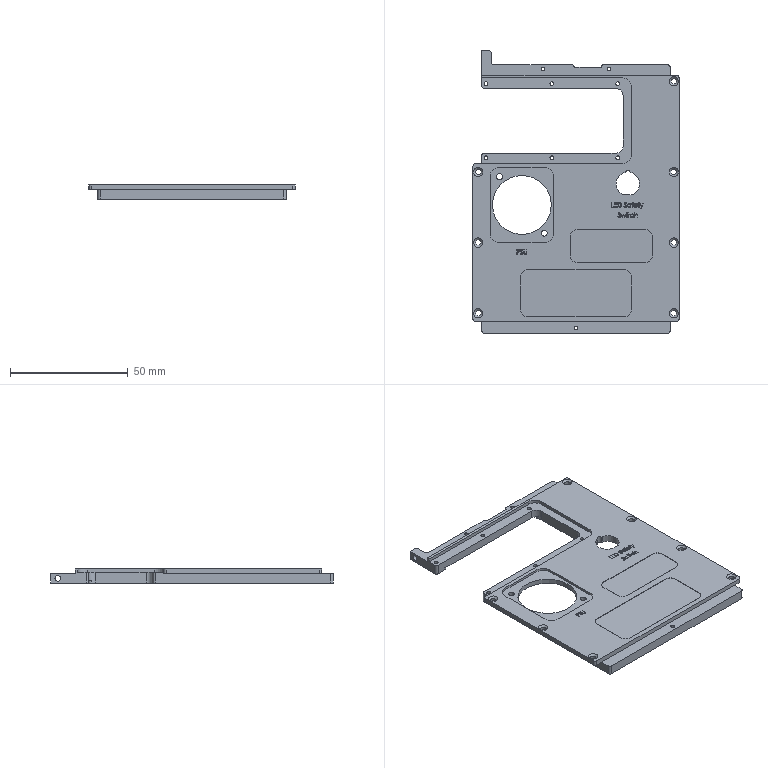NC program | NX | posted with a generic post | part box 87.5 x 120 x 6.001 mm
Whole program:
N10 G17 G21 G94 G90
(PLANAR_MILL_8 , TOOL : D6-18-D6-50-3T-FINISH)
N12 T05 M6
N14 G54
N16 G17 G0 G90 X-15.174 Y-1.985 B0. C0. S5000 M3
N18 G43 Z50. H5
N20 Z-0.75 B-180. C90.
N22 G94 G1 Z-3.75 F300.
N24 G41 X-15. Y-1. D5
N26 Y4.
N28 Y6.
N30 Y11.
N32 G40
N34 X-15.174 Y11.985
N36 Z-0.75
N38 G0 Z50.
N40 M5
(SPOT_DRILLING_3 , TOOL : 点孔D5-120-90度)
N42 T14 M6
N44 G54
N46 G17 G0 G90 X-57. Y2. B0. C0. S2500 M3
N48 G43 Z50. H14
N50 G94 G82 G99 Z-5. B-180. C90. F200. P200 R-0.75
N52 G80
N54 G0 X-57. Y2. Z50.
N56 M5
(SPOT_DRILLING_3_COPY , TOOL : Z2.4)
N58 T15 M6
N60 G54
N62 G17 G0 G90 X-57. Y2. B0. C0. S2500 M3
N64 G43 Z50. H15
N66 G94 G82 G99 Z-9.75 B-180. C90. F200. P200 R-0.75
N68 G80
N70 G0 X-57. Y2. Z50.
N72 M5
N74 M2